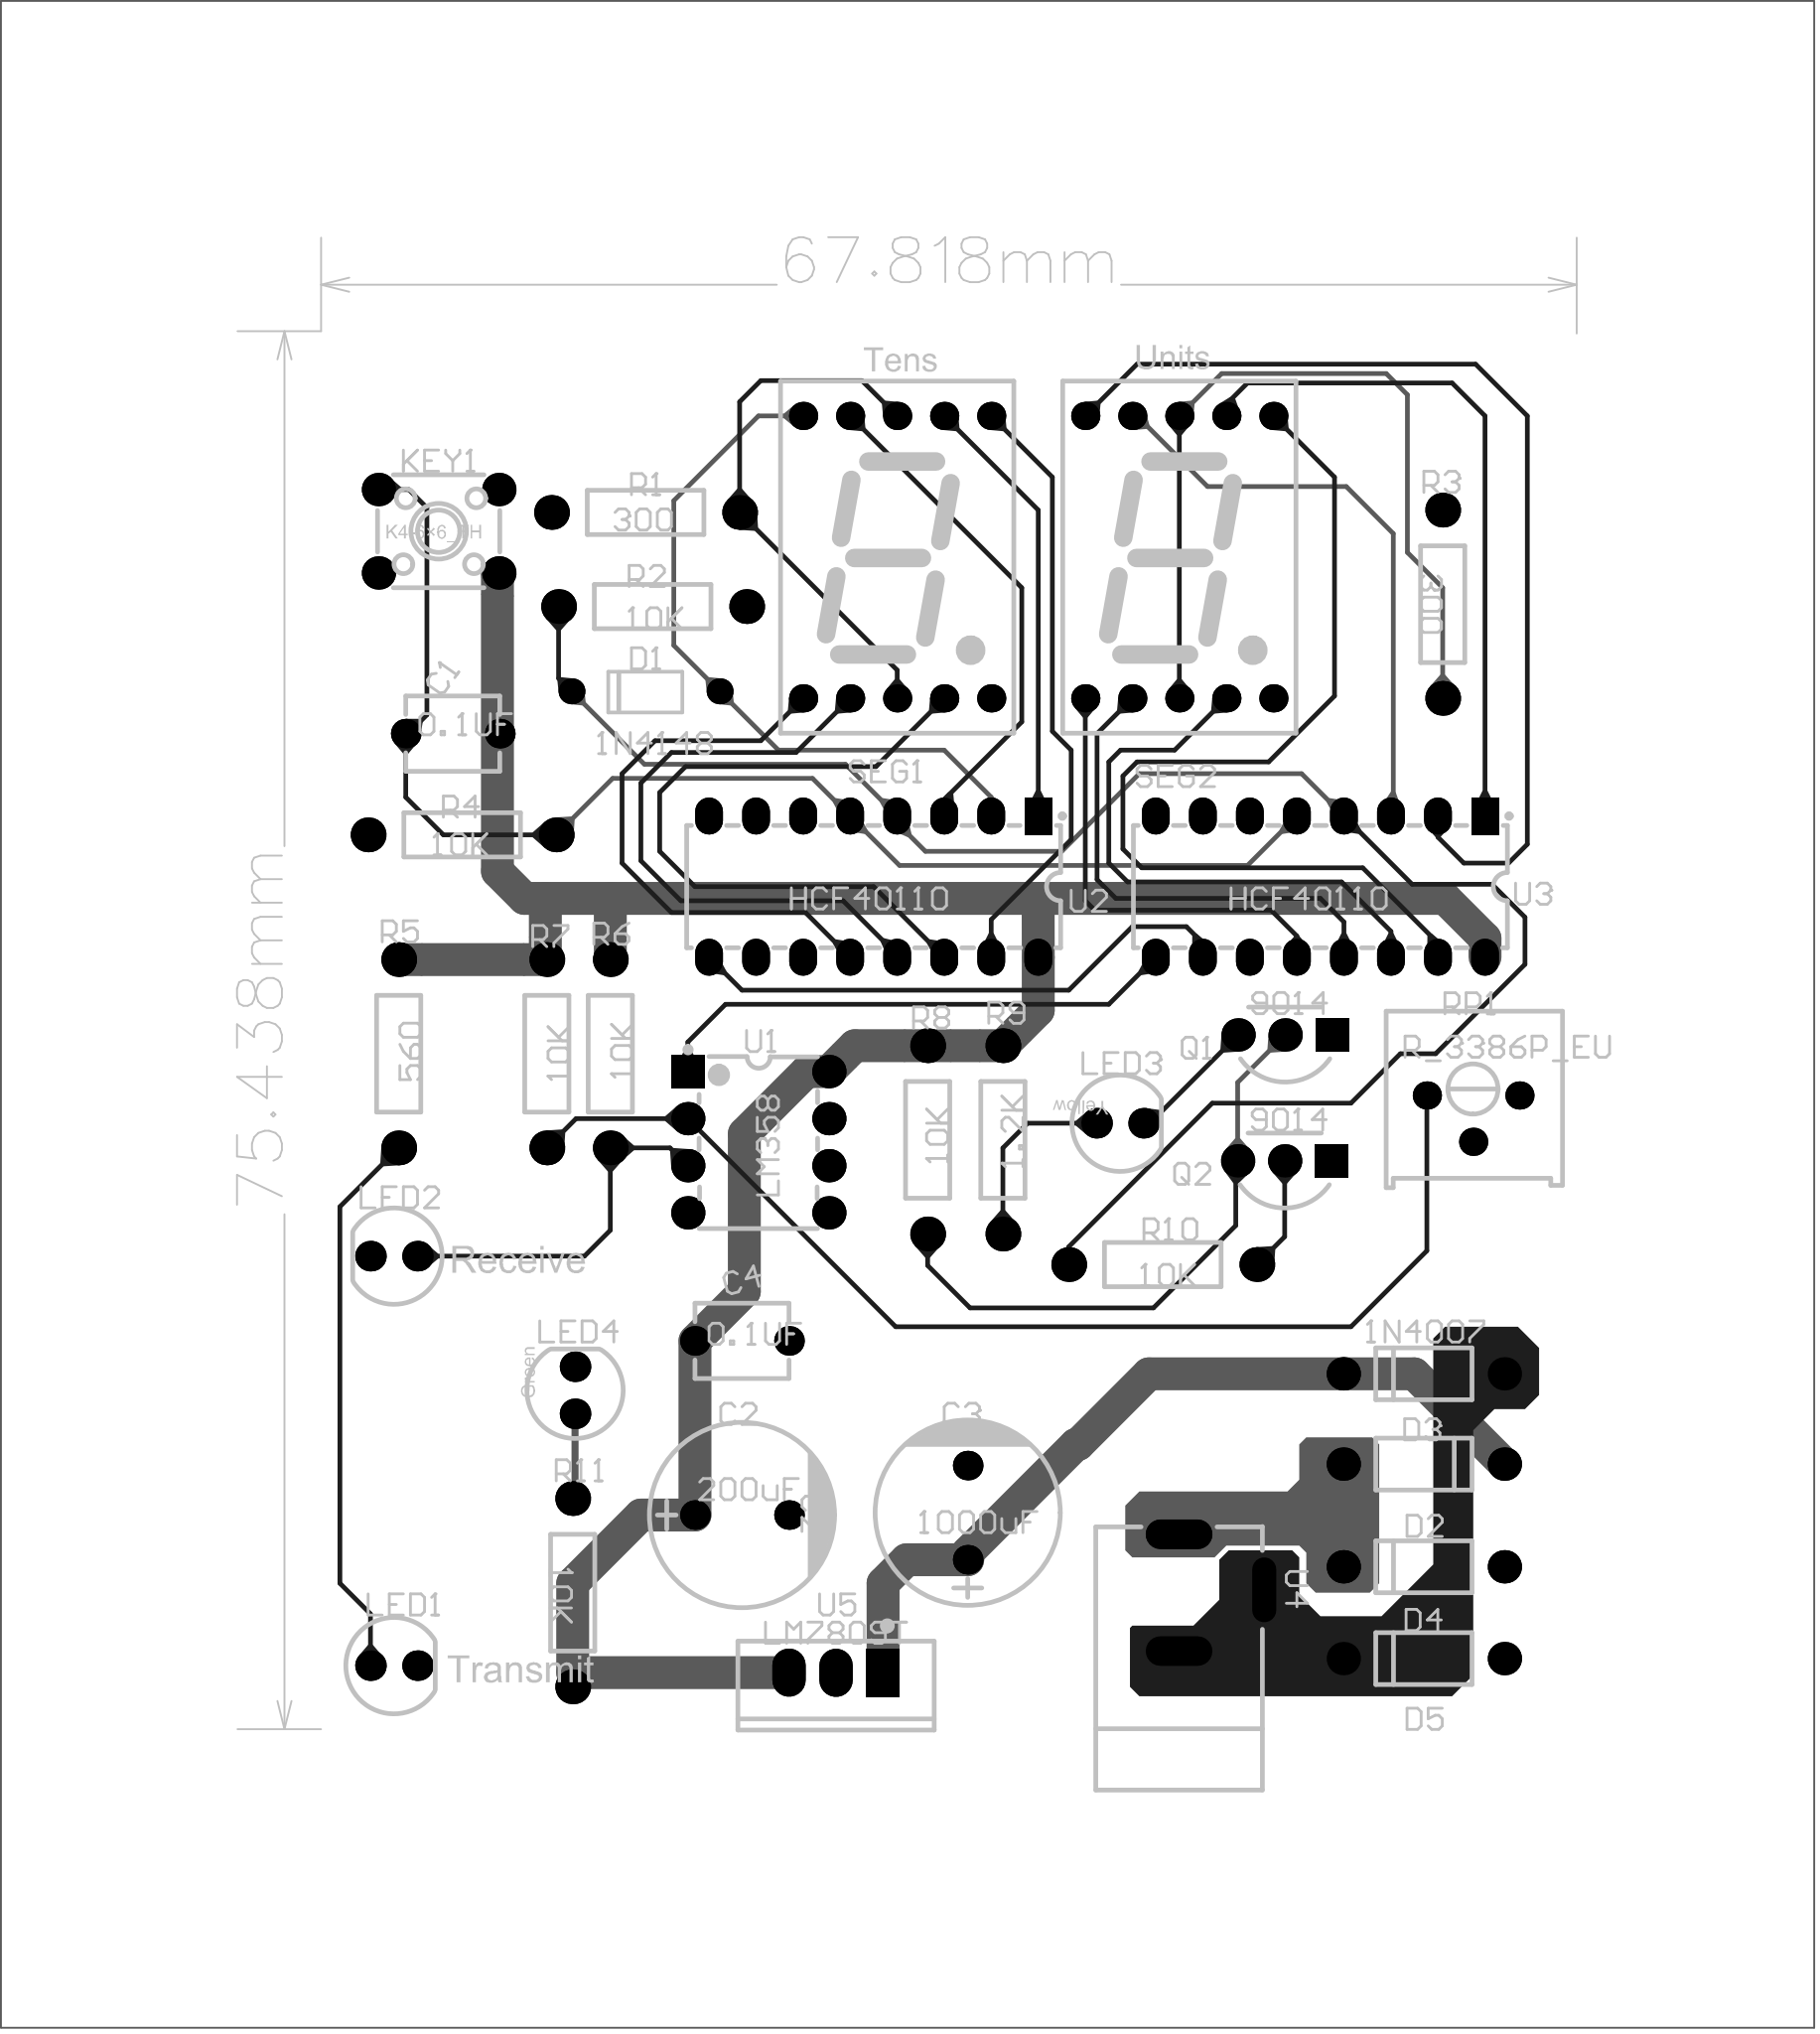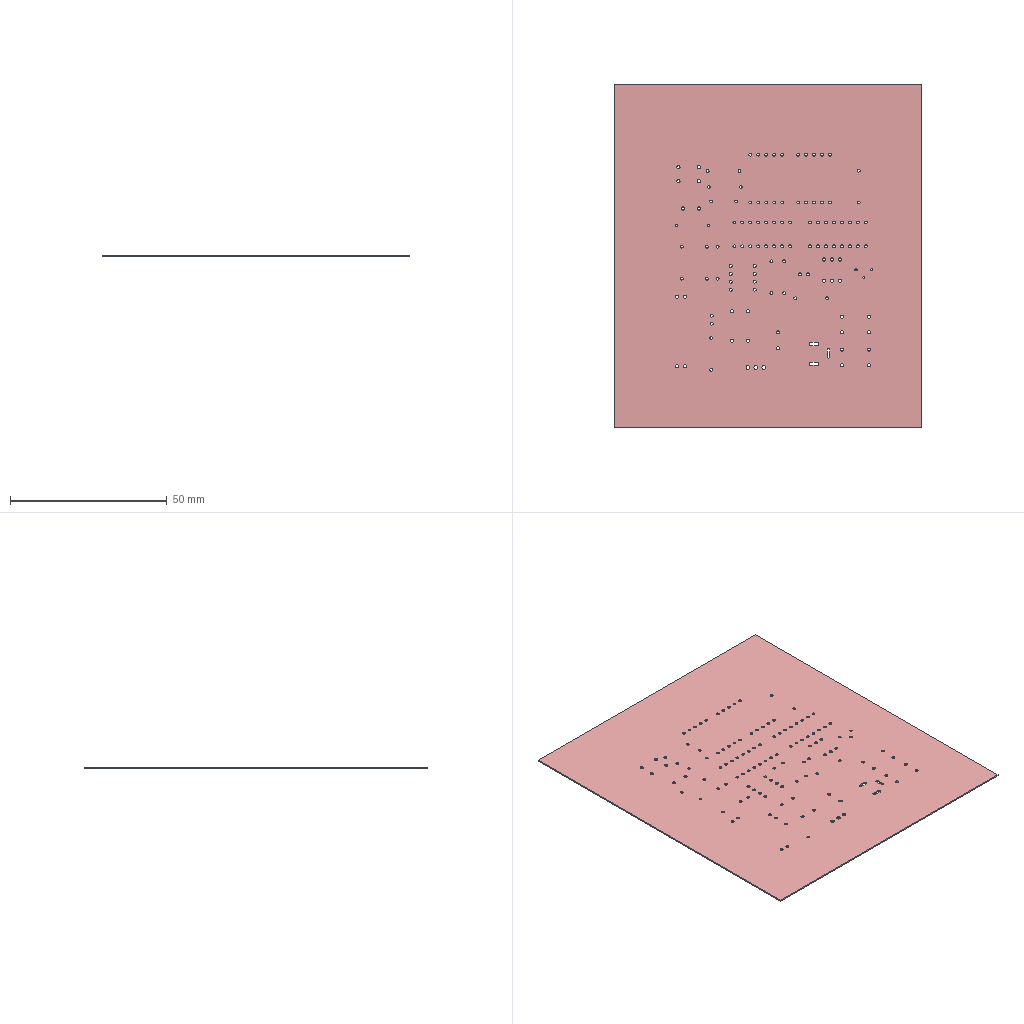Circuit board layout | Altium Designer | box 97.9 x 109.4 x 0.4 mm
Layer stack:
# Altium Designer layer stack of  (unit mm; dielectric type: 0 none, 1 core, 2 prepreg, 3 surface material)
index,name,kind,layer,copper_thickness_mm,dielectric_type,dielectric_thickness_mm,dielectric_material,dielectric_constant
0,Top Solder,dielectric,,,3,0.0102,Solder Resist,3.5
1,Top Paste,other,,,,,,
2,Top Overlay,other,,,,,,
3,Top Layer,copper,Top Layer,0.0356,,,,
4,Dielectric1,dielectric,,,0,0.32,FR-4,4.8
5,Bottom Layer,copper,Bottom Layer,0.0356,,,,
6,Bottom Overlay,other,,,,,,
7,Bottom Paste,other,,,,,,
8,Bottom Solder,dielectric,,,3,0.0102,Solder Resist,3.5
# drill layer pairs: low layer,high layer
drill_pair,Top Layer,Bottom Layer
Part placement:
Designator,Comment,Layer,Footprint,Center-X(mm),Center-Y(mm),Rotation
U5,LM7809T,TopLayer,TO-220-3_L10.0-W4.5-P2.54-L,70.506,44.559,180
U3,HCF40110,TopLayer,DIP-16_16P-L20.2-W6.6-P2.54-LS7.6-BL,96.668,86.977,180
U2,HCF40110,TopLayer,DIP-16_16P-L20.2-W6.6-P2.54-LS7.6-BL,72.537,86.977,180
U1,LM358,TopLayer,DIP-8_L8.8-W6.4-P2.54-LS7.6-BL,66.309,73.187,270
SEG2,SEG-TH_0.56×1_Cathode,TopLayer,LED-SEG-TH_10P-L12.6-W19.0-P2.54-S15.24-BL,89.047,104.757,0
SEG1,SEG-TH_0.56×1_Cathode,TopLayer,LED-SEG-TH_10P-L12.6-W19.0-P2.54-S15.24-BL,73.808,104.757,0
R11,10K,TopLayer,R_AXIAL-0.4,56.282,48.877,270
R10,10K,TopLayer,R_AXIAL-0.4,88.153,66.583,180
R9,1.2K,TopLayer,R_AXIAL-0.4,79.517,73.314,90
R8,10K,TopLayer,R_AXIAL-0.4,75.453,73.314,90
R7,10K,TopLayer,R_AXIAL-0.4,54.885,77.96,90
R6,10K,TopLayer,R_AXIAL-0.4,58.313,77.96,90
R5,560,TopLayer,R_AXIAL-0.4,46.883,77.96,90
R4,10K,TopLayer,R_AXIAL-0.4,50.312,89.771,0
R3,300,TopLayer,R_AXIAL-0.4,103.272,102.217,270
R2,10K,TopLayer,R_AXIAL-0.4,60.599,102.09,0
R1,300,TopLayer,R_AXIAL-0.4,60.218,107.17,0
Q2,9014,TopLayer,TO-92-3_L4.9-W3.7-P2.54-L,94.738,72.179,180
Q1,9014,TopLayer,TO-92-3_L4.9-W3.7-P2.54-L,94.763,78.976,180
LED4,Green,TopLayer,LED-TH_BD5.0_RED,56.408,59.799,180
LED3,Yellow,TopLayer,LED-TH_BD5.0_RED,85.848,74.211,90
LED2,LED-TH-5mm_R,TopLayer,LED-TH_BD5.0_RED,46.63,67.038,270
LED1,LED-TH-5mm_R,TopLayer,LED-TH_BD5.0_RED,46.63,44.94,90
KEY1,K4-6×6_TH,TopLayer,KEY-TH_4P-L6.0-W6.0-P4.50-LS6.5,49.042,106.154,180
D5,1N4007,TopLayer,DO-41_BD2.4-L4.7-P8.70-D0.9-FD,102.255,45.321,180
D4,1N4007,TopLayer,DO-41_BD2.4-L4.7-P8.70-D0.9-FD,102.255,50.274,180
D3,1N4007,TopLayer,DO-41_BD2.4-L4.7-P8.70-D0.9-FD,102.255,60.688,180
D2,1N4007,TopLayer,DO-41_BD2.4-L4.7-P8.70-D0.9-FD,102.255,55.817,0
D1,1N4148,TopLayer,DO-35_BD2.2-L4.0-D0.50_1N4148,60.218,97.518,180
C3,1000uF,TopLayer,CAP-TH_BD10.0-P5.00-D1.0-FD,77.618,53.195,90
C4,0.1UF,TopLayer,CAP-TH_L5.0-W4.0-P5.00-D1.0,65.425,62.466,180
C1,0.1UF,TopLayer,CAP-TH_L5.0-W4.0-P5.00-D1.0,49.804,95.232,0
C2,200uF,TopLayer,CAP-TH_BD10.0-P5.00-D1.0-FD,65.425,53.068,0
U4,HX DC005-2.5,TopLayer,DC-IN-TH_HX-DC005-2.5,91.334,48.877,90
RP1,R_3386P_EU,TopLayer,RES-ADJ-TH_3386P,104.918,74.458,180
,,TopOverlay,,0,0,0
,,TopOverlay,,0,0,0
Pad and via stacks:
# Altium Designer via and pad stacks of  (unit mm). Each distinct definition once, with the count of objects using it.
# via: kind,start_layer,end_layer,hole_mm,diameter_mm,mode(0 simple;1 top-mid-bottom;2 full stack),diameter_per_layer,count,example_net
# pad: kind,layer,hole_mm,hole_type(0 round;1 square;2 slot),plating,top_size,top_shape(1 round;2 rect;3 octagon;9 rounded rect),mid_size,bottom_size,mode,footprint,size_per_layer,count,example
pad,Multi-Layer,1.2,0,plated,1.8x2.6,2,1.8x2.6,1.8x2.6,0,TO-220-3_L10.0-W4.5-P2.54-L,,1,U5.1
pad,Multi-Layer,1.2,0,plated,1.8x2.6,1,1.8x2.6,1.8x2.6,0,TO-220-3_L10.0-W4.5-P2.54-L,,2,U5.3
pad,Multi-Layer,0.9,0,plated,2x1.5,2,2x1.5,2x1.5,0,DIP-16_16P-L20.2-W6.6-P2.54-LS7.6-BL,,2,U3.1
pad,Multi-Layer,0.9,0,plated,2x1.5,1,2x1.5,2x1.5,0,DIP-16_16P-L20.2-W6.6-P2.54-LS7.6-BL,,30,U3.2
pad,Multi-Layer,1,0,plated,1.8x1.8,1,1.8x1.8,1.8x1.8,0,DIP-8_L8.8-W6.4-P2.54-LS7.6-BL,,7,U1.4
pad,Multi-Layer,1,0,plated,1.8x1.8,2,1.8x1.8,1.8x1.8,0,DIP-8_L8.8-W6.4-P2.54-LS7.6-BL,,1,U1.1
pad,Multi-Layer,0.9144,0,plated,1.524x1.524,1,1.524x1.524,1.524x1.524,0,LED-SEG-TH_10P-L12.6-W19.0-P2.54-S15.24-BL,,20,SEG2.10
pad,Multi-Layer,0.8992,0,plated,1.88x1.88,1,1.88x1.88,1.88x1.88,0,R_AXIAL-0.4,,22,R11.2
pad,Multi-Layer,1,0,plated,1.8x1.8,1,1.8x1.8,1.8x1.8,0,TO-92-3_L4.9-W3.7-P2.54-L,,4,Q2.3
pad,Multi-Layer,1,0,plated,1.8x1.8,2,1.8x1.8,1.8x1.8,0,TO-92-3_L4.9-W3.7-P2.54-L,,2,Q2.1
pad,Multi-Layer,0.9652,0,plated,1.651x1.651,1,1.651x1.651,1.651x1.651,0,LED-TH_BD5.0_RED,,8,LED4.2
pad,Multi-Layer,1.1,0,plated,1.8x1.8,1,1.8x1.8,1.8x1.8,0,KEY-TH_4P-L6.0-W6.0-P4.50-LS6.5,,4,KEY1.2
pad,Multi-Layer,1,0,plated,1.8x1.8,1,1.8x1.8,1.8x1.8,0,DO-41_BD2.4-L4.7-P8.70-D0.9-FD,,8,D5.2
pad,Multi-Layer,0.8,0,plated,1.4x1.4,1,1.4x1.4,1.4x1.4,0,DO-35_BD2.2-L4.0-D0.50_1N4148,,2,D1.1
pad,Multi-Layer,1,0,plated,1.6x1.6,1,1.6x1.6,1.6x1.6,0,CAP-TH_BD10.0-P5.00-D1.0-FD,,4,C3.2
pad,Multi-Layer,1,0,plated,1.6x1.6,1,1.6x1.6,1.6x1.6,0,CAP-TH_L5.0-W4.0-P5.00-D1.0,,4,C4.2
pad,Multi-Layer,1,2,plated,1.6x3.6,1,1.6x3.6,1.6x3.6,0,DC-IN-TH_HX-DC005-2.5,,2,U4.3
pad,Multi-Layer,0.8,2,plated,1.3x3.5,1,1.3x3.5,1.3x3.5,0,DC-IN-TH_HX-DC005-2.5,,1,U4.2
pad,Multi-Layer,0.7,0,plated,1.524x1.524,1,1.524x1.524,1.524x1.524,0,RES-ADJ-TH_3386P,,3,RP1.3
Design rules, without the lines most boards share:
# Altium Designer design rules of  (exported by Altium Designer, unit mm)
# columns: name | kind | enabled | priority | scope1 | scope2 | descriptor | typed fields (field=value)
HoleToHoleClearance | 52 | enabled | 1 | All | All | Hole To Hole Clearance (Gap=10mil) (All),(All) | gap=0.254
DiffPairsRouting | 51 | enabled | 1 | All | All | Differential Pairs Uncoupled Length using the Gap Constraints (Min=10mil) (Max=10mil) (Prefered=10mil)  and Width Constraints (Min=15mil) (Max=15mil) (Prefered=15mil) (All) |
SolderMaskExpansion | 13 | enabled | 1 | All | All | Solder Mask Expansion (Expansion =4mil) (All) | expansion=0.1016
PasteMaskExpansion | 14 | enabled | 1 | All | All | Paste Mask Expansion (Expansion =0mil) (All) | expansion=0
RoutingVias | 11 | enabled | 1 | All | All | Routing Via (MinHoleWidth=28mil) (MaxHoleWidth=28mil) (PreferredHoleWidth=28mil) (MinWidth=50mil) (MaxWidth=50mil) (PreferedWidth=50mil) (All) | via_min_hole=0.7112 via_max_hole=0.7112 via_preferred_diameter=1.27 via_preferred_hole=0.7112
Width | 2 | enabled | 1 | All | All | Width Constraint (Min=10mil) (Max=10mil) (Preferred=10mil) (All) |
PolygonConnect | 20 | enabled | 1 | All | All | Polygon Connect Rule(Relief Connect )(Conductor Width=10mil) (Relief Angle=90 Angle) (Entries=4) (Air Gap Width=10mil) (All),(All) | connect_style(0=relief,1=direct,2=none)=0 relief_conductor_width=0.254 relief_entries=4
PlaneConnect | 6 | enabled | 1 | All | All | Power Plane Connect Rule(Relief Connect )(Expansion=20mil) (Conductor Width=10mil) (Air Gap=10mil) (Entries=4) (All) | relief_conductor_width=0.254 relief_entries=4 relief_expansion=0.508
Clearance | 0 | enabled | 1 | All | All | Clearance Constraint (Gap=10mil) (All),(All) | gap=0.254